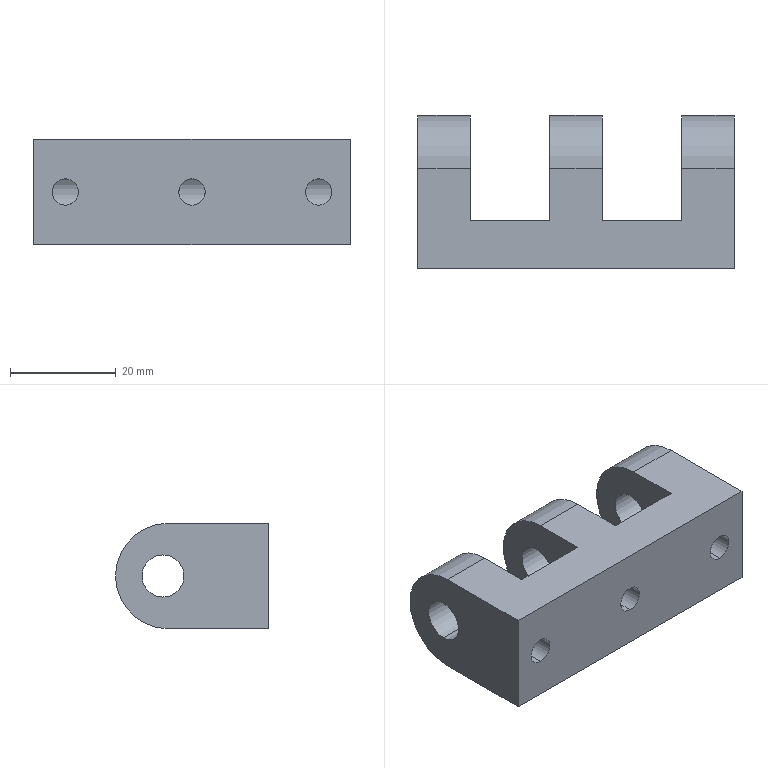Part | SolidWorks | features BaseBody 1 | 1 solid | 26 faces | box 60 x 29 x 20 mm | volume 19050 mm3 | cylinder 15 | plane 11 | commonest cylinder face diameters 5 x6 8 x6 20 x3
STEP:
#1=CARTESIAN_POINT('',(-24.,16.878,-2.5));
#2=VERTEX_POINT('',#1);
#3=CARTESIAN_POINT('',(-24.,16.878,2.5));
#4=VERTEX_POINT('',#3);
#5=CARTESIAN_POINT('',(-24.,16.878,-2.5));
#6=CARTESIAN_POINT('',(-24.17,16.878,-2.5));
#7=CARTESIAN_POINT('',(-24.337,16.864,-2.483));
#8=CARTESIAN_POINT('',(-24.662,16.812,-2.417));
#9=CARTESIAN_POINT('',(-24.822,16.774,-2.367));
#10=CARTESIAN_POINT('',(-25.27,16.641,-2.178));
#11=CARTESIAN_POINT('',(-25.539,16.524,-1.996));
#12=CARTESIAN_POINT('',(-25.876,16.358,-1.66));
#13=CARTESIAN_POINT('',(-25.98,16.304,-1.535));
#14=CARTESIAN_POINT('',(-26.16,16.204,-1.269));
#15=CARTESIAN_POINT('',(-26.237,16.159,-1.128));
#16=CARTESIAN_POINT('',(-26.365,16.083,-0.8272));
#17=CARTESIAN_POINT('',(-26.415,16.052,-0.6657));
#18=CARTESIAN_POINT('',(-26.482,16.011,-0.3399));
#19=CARTESIAN_POINT('',(-26.5,16.,-0.1739));
#20=CARTESIAN_POINT('',(-26.5,16.,0.1647));
#21=CARTESIAN_POINT('',(-26.483,16.011,0.3339));
#22=CARTESIAN_POINT('',(-26.417,16.052,0.6609));
#23=CARTESIAN_POINT('',(-26.367,16.082,0.8221));
#24=CARTESIAN_POINT('',(-26.175,16.196,1.276));
#25=CARTESIAN_POINT('',(-25.989,16.303,1.547));
#26=CARTESIAN_POINT('',(-25.652,16.469,1.883));
#27=CARTESIAN_POINT('',(-25.527,16.526,1.986));
#28=CARTESIAN_POINT('',(-25.262,16.634,2.164));
#29=CARTESIAN_POINT('',(-25.122,16.685,2.24));
#30=CARTESIAN_POINT('',(-24.823,16.774,2.366));
#31=CARTESIAN_POINT('',(-24.663,16.812,2.416));
#32=CARTESIAN_POINT('',(-24.337,16.863,2.483));
#33=CARTESIAN_POINT('',(-24.171,16.878,2.5));
#34=CARTESIAN_POINT('',(-24.,16.878,2.5));
#35=B_SPLINE_CURVE_WITH_KNOTS('',3,(#5,#6,#7,#8,#9,#10,#11,#12,#13,#14,#15,#16,#17,#18,#19,#20,#21,#22,#23,#24,#25,#26,#27,#28,#29,#30,#31,#32,#33,#34),.UNSPECIFIED.,.F.,.F.,(4,2,2,2,2,2,2,2,2,2,2,2,2,2,4),(0.,0.0005024,0.001005,0.00201,0.002512,0.003015,0.003517,0.004019,0.004522,0.005024,0.006029,0.006532,0.007034,0.007536,0.008039),.UNSPECIFIED.);
#36=EDGE_CURVE('',#2,#4,#35,.T.);
#37=ORIENTED_EDGE('',*,*,#36,.F.);
#38=CARTESIAN_POINT('',(-24.,16.878,2.5));
#39=CARTESIAN_POINT('',(-23.83,16.878,2.5));
#40=CARTESIAN_POINT('',(-23.663,16.864,2.483));
#41=CARTESIAN_POINT('',(-23.338,16.812,2.417));
#42=CARTESIAN_POINT('',(-23.178,16.774,2.367));
#43=CARTESIAN_POINT('',(-22.73,16.641,2.178));
#44=CARTESIAN_POINT('',(-22.461,16.524,1.996));
#45=CARTESIAN_POINT('',(-22.124,16.358,1.66));
#46=CARTESIAN_POINT('',(-22.02,16.304,1.535));
#47=CARTESIAN_POINT('',(-21.84,16.204,1.269));
#48=CARTESIAN_POINT('',(-21.763,16.159,1.128));
#49=CARTESIAN_POINT('',(-21.635,16.083,0.8272));
#50=CARTESIAN_POINT('',(-21.585,16.052,0.6657));
#51=CARTESIAN_POINT('',(-21.518,16.011,0.3399));
#52=CARTESIAN_POINT('',(-21.5,16.,0.1739));
#53=CARTESIAN_POINT('',(-21.5,16.,-0.1647));
#54=CARTESIAN_POINT('',(-21.517,16.011,-0.3339));
#55=CARTESIAN_POINT('',(-21.583,16.052,-0.6609));
#56=CARTESIAN_POINT('',(-21.633,16.082,-0.8221));
#57=CARTESIAN_POINT('',(-21.825,16.196,-1.276));
#58=CARTESIAN_POINT('',(-22.011,16.303,-1.547));
#59=CARTESIAN_POINT('',(-22.348,16.469,-1.883));
#60=CARTESIAN_POINT('',(-22.473,16.526,-1.986));
#61=CARTESIAN_POINT('',(-22.738,16.634,-2.164));
#62=CARTESIAN_POINT('',(-22.878,16.685,-2.24));
#63=CARTESIAN_POINT('',(-23.177,16.774,-2.366));
#64=CARTESIAN_POINT('',(-23.337,16.812,-2.416));
#65=CARTESIAN_POINT('',(-23.663,16.863,-2.483));
#66=CARTESIAN_POINT('',(-23.83,16.878,-2.5));
#67=CARTESIAN_POINT('',(-24.,16.878,-2.5));
#68=B_SPLINE_CURVE_WITH_KNOTS('',3,(#38,#39,#40,#41,#42,#43,#44,#45,#46,#47,#48,#49,#50,#51,#52,#53,#54,#55,#56,#57,#58,#59,#60,#61,#62,#63,#64,#65,#66,#67),.UNSPECIFIED.,.F.,.F.,(4,2,2,2,2,2,2,2,2,2,2,2,2,2,4),(0.008039,0.00854,0.009042,0.01004,0.01055,0.01105,0.01155,0.01205,0.01255,0.01305,0.01406,0.01456,0.01506,0.01556,0.01606),.UNSPECIFIED.);
#69=EDGE_CURVE('',#4,#2,#68,.T.);
#70=ORIENTED_EDGE('',*,*,#69,.F.);
#71=EDGE_LOOP('',(#37,#70));
#72=FACE_BOUND('',#71,.T.);
#73=CARTESIAN_POINT('',(-30.,20.,4.));
#74=VERTEX_POINT('',#73);
#75=CARTESIAN_POINT('',(-30.,20.,-4.));
#76=VERTEX_POINT('',#75);
#77=CARTESIAN_POINT('',(-30.,20.,0.));
#78=DIRECTION('',(1.,0.,0.));
#79=DIRECTION('',(0.,0.,-1.));
#80=AXIS2_PLACEMENT_3D('',#77,#78,#79);
#81=CIRCLE('',#80,4.);
#82=EDGE_CURVE('',#74,#76,#81,.T.);
#83=ORIENTED_EDGE('',*,*,#82,.F.);
#84=CARTESIAN_POINT('',(-20.,20.,4.));
#85=VERTEX_POINT('',#84);
#86=CARTESIAN_POINT('',(-30.,20.,4.));
#87=DIRECTION('',(1.,0.,0.));
#88=VECTOR('',#87,1000.);
#89=LINE('',#86,#88);
#90=EDGE_CURVE('',#74,#85,#89,.T.);
#91=ORIENTED_EDGE('',*,*,#90,.T.);
#92=CARTESIAN_POINT('',(-20.,20.,-4.));
#93=VERTEX_POINT('',#92);
#94=CARTESIAN_POINT('',(-20.,20.,0.));
#95=DIRECTION('',(-1.,0.,0.));
#96=DIRECTION('',(0.,0.,1.));
#97=AXIS2_PLACEMENT_3D('',#94,#95,#96);
#98=CIRCLE('',#97,4.);
#99=EDGE_CURVE('',#93,#85,#98,.T.);
#100=ORIENTED_EDGE('',*,*,#99,.F.);
#101=CARTESIAN_POINT('',(-30.,20.,-4.));
#102=DIRECTION('',(1.,0.,0.));
#103=VECTOR('',#102,1000.);
#104=LINE('',#101,#103);
#105=EDGE_CURVE('',#76,#93,#104,.T.);
#106=ORIENTED_EDGE('',*,*,#105,.F.);
#107=EDGE_LOOP('',(#83,#91,#100,#106));
#108=FACE_OUTER_BOUND('',#107,.T.);
#109=CARTESIAN_POINT('',(-30.,20.,0.));
#110=DIRECTION('',(1.,0.,0.));
#111=DIRECTION('',(0.,0.,-1.));
#112=AXIS2_PLACEMENT_3D('',#109,#110,#111);
#113=CYLINDRICAL_SURFACE('',#112,4.);
#114=ADVANCED_FACE('',(#72,#108),#113,.F.);
#115=CARTESIAN_POINT('',(0.,16.878,-2.5));
#116=VERTEX_POINT('',#115);
#117=CARTESIAN_POINT('',(0.,16.878,2.5));
#118=VERTEX_POINT('',#117);
#119=CARTESIAN_POINT('',(0.,16.878,-2.5));
#120=CARTESIAN_POINT('',(-0.1704,16.878,-2.5));
#121=CARTESIAN_POINT('',(-0.3367,16.864,-2.483));
#122=CARTESIAN_POINT('',(-0.6617,16.812,-2.417));
#123=CARTESIAN_POINT('',(-0.8216,16.774,-2.367));
#124=CARTESIAN_POINT('',(-1.27,16.641,-2.178));
#125=CARTESIAN_POINT('',(-1.539,16.524,-1.996));
#126=CARTESIAN_POINT('',(-1.876,16.358,-1.66));
#127=CARTESIAN_POINT('',(-1.98,16.304,-1.535));
#128=CARTESIAN_POINT('',(-2.16,16.204,-1.269));
#129=CARTESIAN_POINT('',(-2.237,16.159,-1.128));
#130=CARTESIAN_POINT('',(-2.365,16.083,-0.8272));
#131=CARTESIAN_POINT('',(-2.415,16.052,-0.6657));
#132=CARTESIAN_POINT('',(-2.482,16.011,-0.3399));
#133=CARTESIAN_POINT('',(-2.5,16.,-0.1739));
#134=CARTESIAN_POINT('',(-2.5,16.,0.1647));
#135=CARTESIAN_POINT('',(-2.483,16.011,0.3339));
#136=CARTESIAN_POINT('',(-2.417,16.052,0.6609));
#137=CARTESIAN_POINT('',(-2.367,16.082,0.8221));
#138=CARTESIAN_POINT('',(-2.175,16.196,1.276));
#139=CARTESIAN_POINT('',(-1.989,16.303,1.547));
#140=CARTESIAN_POINT('',(-1.652,16.469,1.883));
#141=CARTESIAN_POINT('',(-1.527,16.526,1.986));
#142=CARTESIAN_POINT('',(-1.262,16.634,2.164));
#143=CARTESIAN_POINT('',(-1.122,16.685,2.24));
#144=CARTESIAN_POINT('',(-0.8234,16.774,2.366));
#145=CARTESIAN_POINT('',(-0.6631,16.812,2.416));
#146=CARTESIAN_POINT('',(-0.3373,16.863,2.483));
#147=CARTESIAN_POINT('',(-0.1708,16.878,2.5));
#148=CARTESIAN_POINT('',(0.,16.878,2.5));
#149=B_SPLINE_CURVE_WITH_KNOTS('',3,(#119,#120,#121,#122,#123,#124,#125,#126,#127,#128,#129,#130,#131,#132,#133,#134,#135,#136,#137,#138,#139,#140,#141,#142,#143,#144,#145,#146,#147,#148),.UNSPECIFIED.,.F.,.F.,(4,2,2,2,2,2,2,2,2,2,2,2,2,2,4),(0.,0.0005024,0.001005,0.00201,0.002512,0.003015,0.003517,0.004019,0.004522,0.005024,0.006029,0.006532,0.007034,0.007536,0.008039),.UNSPECIFIED.);
#150=EDGE_CURVE('',#116,#118,#149,.T.);
#151=ORIENTED_EDGE('',*,*,#150,.F.);
#152=CARTESIAN_POINT('',(0.,16.878,2.5));
#153=CARTESIAN_POINT('',(0.1704,16.878,2.5));
#154=CARTESIAN_POINT('',(0.3367,16.864,2.483));
#155=CARTESIAN_POINT('',(0.6617,16.812,2.417));
#156=CARTESIAN_POINT('',(0.8216,16.774,2.367));
#157=CARTESIAN_POINT('',(1.27,16.641,2.178));
#158=CARTESIAN_POINT('',(1.539,16.524,1.996));
#159=CARTESIAN_POINT('',(1.876,16.358,1.66));
#160=CARTESIAN_POINT('',(1.98,16.304,1.535));
#161=CARTESIAN_POINT('',(2.16,16.204,1.269));
#162=CARTESIAN_POINT('',(2.237,16.159,1.128));
#163=CARTESIAN_POINT('',(2.365,16.083,0.8272));
#164=CARTESIAN_POINT('',(2.415,16.052,0.6657));
#165=CARTESIAN_POINT('',(2.482,16.011,0.3399));
#166=CARTESIAN_POINT('',(2.5,16.,0.1739));
#167=CARTESIAN_POINT('',(2.5,16.,-0.1647));
#168=CARTESIAN_POINT('',(2.483,16.011,-0.3339));
#169=CARTESIAN_POINT('',(2.417,16.052,-0.6609));
#170=CARTESIAN_POINT('',(2.367,16.082,-0.8221));
#171=CARTESIAN_POINT('',(2.175,16.196,-1.276));
#172=CARTESIAN_POINT('',(1.989,16.303,-1.547));
#173=CARTESIAN_POINT('',(1.652,16.469,-1.883));
#174=CARTESIAN_POINT('',(1.527,16.526,-1.986));
#175=CARTESIAN_POINT('',(1.262,16.634,-2.164));
#176=CARTESIAN_POINT('',(1.122,16.685,-2.24));
#177=CARTESIAN_POINT('',(0.8234,16.774,-2.366));
#178=CARTESIAN_POINT('',(0.6631,16.812,-2.416));
#179=CARTESIAN_POINT('',(0.3373,16.863,-2.483));
#180=CARTESIAN_POINT('',(0.1701,16.878,-2.5));
#181=CARTESIAN_POINT('',(0.,16.878,-2.5));
#182=B_SPLINE_CURVE_WITH_KNOTS('',3,(#152,#153,#154,#155,#156,#157,#158,#159,#160,#161,#162,#163,#164,#165,#166,#167,#168,#169,#170,#171,#172,#173,#174,#175,#176,#177,#178,#179,#180,#181),.UNSPECIFIED.,.F.,.F.,(4,2,2,2,2,2,2,2,2,2,2,2,2,2,4),(0.008039,0.00854,0.009042,0.01004,0.01055,0.01105,0.01155,0.01205,0.01255,0.01305,0.01406,0.01456,0.01506,0.01556,0.01606),.UNSPECIFIED.);
#183=EDGE_CURVE('',#118,#116,#182,.T.);
#184=ORIENTED_EDGE('',*,*,#183,.F.);
#185=EDGE_LOOP('',(#151,#184));
#186=FACE_BOUND('',#185,.T.);
#187=CARTESIAN_POINT('',(-5.,20.,4.));
#188=VERTEX_POINT('',#187);
#189=CARTESIAN_POINT('',(-5.,20.,-4.));
#190=VERTEX_POINT('',#189);
#191=CARTESIAN_POINT('',(-5.,20.,0.));
#192=DIRECTION('',(1.,0.,0.));
#193=DIRECTION('',(0.,1.,0.));
#194=AXIS2_PLACEMENT_3D('',#191,#192,#193);
#195=CIRCLE('',#194,4.);
#196=EDGE_CURVE('',#188,#190,#195,.T.);
#197=ORIENTED_EDGE('',*,*,#196,.F.);
#198=CARTESIAN_POINT('',(5.,20.,4.));
#199=VERTEX_POINT('',#198);
#200=CARTESIAN_POINT('',(-30.,20.,4.));
#201=DIRECTION('',(1.,0.,0.));
#202=VECTOR('',#201,1000.);
#203=LINE('',#200,#202);
#204=EDGE_CURVE('',#188,#199,#203,.T.);
#205=ORIENTED_EDGE('',*,*,#204,.T.);
#206=CARTESIAN_POINT('',(5.,20.,-4.));
#207=VERTEX_POINT('',#206);
#208=CARTESIAN_POINT('',(5.,20.,0.));
#209=DIRECTION('',(-1.,0.,0.));
#210=DIRECTION('',(0.,0.,1.));
#211=AXIS2_PLACEMENT_3D('',#208,#209,#210);
#212=CIRCLE('',#211,4.);
#213=EDGE_CURVE('',#207,#199,#212,.T.);
#214=ORIENTED_EDGE('',*,*,#213,.F.);
#215=CARTESIAN_POINT('',(-30.,20.,-4.));
#216=DIRECTION('',(1.,0.,0.));
#217=VECTOR('',#216,1000.);
#218=LINE('',#215,#217);
#219=EDGE_CURVE('',#190,#207,#218,.T.);
#220=ORIENTED_EDGE('',*,*,#219,.F.);
#221=EDGE_LOOP('',(#197,#205,#214,#220));
#222=FACE_OUTER_BOUND('',#221,.T.);
#223=CARTESIAN_POINT('',(-30.,20.,0.));
#224=DIRECTION('',(1.,0.,0.));
#225=DIRECTION('',(0.,0.,-1.));
#226=AXIS2_PLACEMENT_3D('',#223,#224,#225);
#227=CYLINDRICAL_SURFACE('',#226,4.);
#228=ADVANCED_FACE('',(#186,#222),#227,.F.);
#229=CARTESIAN_POINT('',(24.,16.878,-2.5));
#230=VERTEX_POINT('',#229);
#231=CARTESIAN_POINT('',(24.,16.878,2.5));
#232=VERTEX_POINT('',#231);
#233=CARTESIAN_POINT('',(24.,16.878,-2.5));
#234=CARTESIAN_POINT('',(23.83,16.878,-2.5));
#235=CARTESIAN_POINT('',(23.663,16.864,-2.483));
#236=CARTESIAN_POINT('',(23.338,16.812,-2.417));
#237=CARTESIAN_POINT('',(23.178,16.774,-2.367));
#238=CARTESIAN_POINT('',(22.73,16.641,-2.178));
#239=CARTESIAN_POINT('',(22.461,16.524,-1.996));
#240=CARTESIAN_POINT('',(22.124,16.358,-1.66));
#241=CARTESIAN_POINT('',(22.02,16.304,-1.535));
#242=CARTESIAN_POINT('',(21.84,16.204,-1.269));
#243=CARTESIAN_POINT('',(21.763,16.159,-1.128));
#244=CARTESIAN_POINT('',(21.635,16.083,-0.8272));
#245=CARTESIAN_POINT('',(21.585,16.052,-0.6657));
#246=CARTESIAN_POINT('',(21.518,16.011,-0.3399));
#247=CARTESIAN_POINT('',(21.5,16.,-0.1739));
#248=CARTESIAN_POINT('',(21.5,16.,0.1647));
#249=CARTESIAN_POINT('',(21.517,16.011,0.3339));
#250=CARTESIAN_POINT('',(21.583,16.052,0.6609));
#251=CARTESIAN_POINT('',(21.633,16.082,0.8221));
#252=CARTESIAN_POINT('',(21.825,16.196,1.276));
#253=CARTESIAN_POINT('',(22.011,16.303,1.547));
#254=CARTESIAN_POINT('',(22.348,16.469,1.883));
#255=CARTESIAN_POINT('',(22.473,16.526,1.986));
#256=CARTESIAN_POINT('',(22.738,16.634,2.164));
#257=CARTESIAN_POINT('',(22.878,16.685,2.24));
#258=CARTESIAN_POINT('',(23.177,16.774,2.366));
#259=CARTESIAN_POINT('',(23.337,16.812,2.416));
#260=CARTESIAN_POINT('',(23.663,16.863,2.483));
#261=CARTESIAN_POINT('',(23.829,16.878,2.5));
#262=CARTESIAN_POINT('',(24.,16.878,2.5));
#263=B_SPLINE_CURVE_WITH_KNOTS('',3,(#233,#234,#235,#236,#237,#238,#239,#240,#241,#242,#243,#244,#245,#246,#247,#248,#249,#250,#251,#252,#253,#254,#255,#256,#257,#258,#259,#260,#261,#262),.UNSPECIFIED.,.F.,.F.,(4,2,2,2,2,2,2,2,2,2,2,2,2,2,4),(0.,0.0005024,0.001005,0.00201,0.002512,0.003015,0.003517,0.004019,0.004522,0.005024,0.006029,0.006532,0.007034,0.007536,0.008039),.UNSPECIFIED.);
#264=EDGE_CURVE('',#230,#232,#263,.T.);
#265=ORIENTED_EDGE('',*,*,#264,.F.);
#266=CARTESIAN_POINT('',(24.,16.878,2.5));
#267=CARTESIAN_POINT('',(24.17,16.878,2.5));
#268=CARTESIAN_POINT('',(24.337,16.864,2.483));
#269=CARTESIAN_POINT('',(24.662,16.812,2.417));
#270=CARTESIAN_POINT('',(24.822,16.774,2.367));
#271=CARTESIAN_POINT('',(25.27,16.641,2.178));
#272=CARTESIAN_POINT('',(25.539,16.524,1.996));
#273=CARTESIAN_POINT('',(25.876,16.358,1.66));
#274=CARTESIAN_POINT('',(25.98,16.304,1.535));
#275=CARTESIAN_POINT('',(26.16,16.204,1.269));
#276=CARTESIAN_POINT('',(26.237,16.159,1.128));
#277=CARTESIAN_POINT('',(26.365,16.083,0.8272));
#278=CARTESIAN_POINT('',(26.415,16.052,0.6657));
#279=CARTESIAN_POINT('',(26.482,16.011,0.3399));
#280=CARTESIAN_POINT('',(26.5,16.,0.1739));
#281=CARTESIAN_POINT('',(26.5,16.,-0.1647));
#282=CARTESIAN_POINT('',(26.483,16.011,-0.3339));
#283=CARTESIAN_POINT('',(26.417,16.052,-0.6609));
#284=CARTESIAN_POINT('',(26.367,16.082,-0.8221));
#285=CARTESIAN_POINT('',(26.175,16.196,-1.276));
#286=CARTESIAN_POINT('',(25.989,16.303,-1.547));
#287=CARTESIAN_POINT('',(25.652,16.469,-1.883));
#288=CARTESIAN_POINT('',(25.527,16.526,-1.986));
#289=CARTESIAN_POINT('',(25.262,16.634,-2.164));
#290=CARTESIAN_POINT('',(25.122,16.685,-2.24));
#291=CARTESIAN_POINT('',(24.823,16.774,-2.366));
#292=CARTESIAN_POINT('',(24.663,16.812,-2.416));
#293=CARTESIAN_POINT('',(24.337,16.863,-2.483));
#294=CARTESIAN_POINT('',(24.17,16.878,-2.5));
#295=CARTESIAN_POINT('',(24.,16.878,-2.5));
#296=B_SPLINE_CURVE_WITH_KNOTS('',3,(#266,#267,#268,#269,#270,#271,#272,#273,#274,#275,#276,#277,#278,#279,#280,#281,#282,#283,#284,#285,#286,#287,#288,#289,#290,#291,#292,#293,#294,#295),.UNSPECIFIED.,.F.,.F.,(4,2,2,2,2,2,2,2,2,2,2,2,2,2,4),(0.008039,0.00854,0.009042,0.01004,0.01055,0.01105,0.01155,0.01205,0.01255,0.01305,0.01406,0.01456,0.01506,0.01556,0.01606),.UNSPECIFIED.);
#297=EDGE_CURVE('',#232,#230,#296,.T.);
#298=ORIENTED_EDGE('',*,*,#297,.F.);
#299=EDGE_LOOP('',(#265,#298));
#300=FACE_BOUND('',#299,.T.);
#301=CARTESIAN_POINT('',(20.,20.,4.));
#302=VERTEX_POINT('',#301);
#303=CARTESIAN_POINT('',(20.,20.,-4.));
#304=VERTEX_POINT('',#303);
#305=CARTESIAN_POINT('',(20.,20.,0.));
#306=DIRECTION('',(1.,0.,0.));
#307=DIRECTION('',(0.,1.,0.));
#308=AXIS2_PLACEMENT_3D('',#305,#306,#307);
#309=CIRCLE('',#308,4.);
#310=EDGE_CURVE('',#302,#304,#309,.T.);
#311=ORIENTED_EDGE('',*,*,#310,.F.);
#312=CARTESIAN_POINT('',(30.,20.,4.));
#313=VERTEX_POINT('',#312);
#314=CARTESIAN_POINT('',(-30.,20.,4.));
#315=DIRECTION('',(1.,0.,0.));
#316=VECTOR('',#315,1000.);
#317=LINE('',#314,#316);
#318=EDGE_CURVE('',#302,#313,#317,.T.);
#319=ORIENTED_EDGE('',*,*,#318,.T.);
#320=CARTESIAN_POINT('',(30.,20.,-4.));
#321=VERTEX_POINT('',#320);
#322=CARTESIAN_POINT('',(30.,20.,0.));
#323=DIRECTION('',(1.,0.,0.));
#324=DIRECTION('',(0.,0.,-1.));
#325=AXIS2_PLACEMENT_3D('',#322,#323,#324);
#326=CIRCLE('',#325,4.);
#327=EDGE_CURVE('',#313,#321,#326,.T.);
#328=ORIENTED_EDGE('',*,*,#327,.T.);
#329=CARTESIAN_POINT('',(-30.,20.,-4.));
#330=DIRECTION('',(1.,0.,0.));
#331=VECTOR('',#330,1000.);
#332=LINE('',#329,#331);
#333=EDGE_CURVE('',#304,#321,#332,.T.);
#334=ORIENTED_EDGE('',*,*,#333,.F.);
#335=EDGE_LOOP('',(#311,#319,#328,#334));
#336=FACE_OUTER_BOUND('',#335,.T.);
#337=CARTESIAN_POINT('',(-30.,20.,0.));
#338=DIRECTION('',(1.,0.,0.));
#339=DIRECTION('',(0.,0.,-1.));
#340=AXIS2_PLACEMENT_3D('',#337,#338,#339);
#341=CYLINDRICAL_SURFACE('',#340,4.);
#342=ADVANCED_FACE('',(#300,#336),#341,.F.);
#343=ORIENTED_EDGE('',*,*,#36,.T.);
#344=CARTESIAN_POINT('',(-24.,0.,2.5));
#345=VERTEX_POINT('',#344);
#346=CARTESIAN_POINT('',(-24.,0.,2.5));
#347=DIRECTION('',(0.,-1.,0.));
#348=VECTOR('',#347,1000.);
#349=LINE('',#346,#348);
#350=EDGE_CURVE('',#4,#345,#349,.T.);
#351=ORIENTED_EDGE('',*,*,#350,.T.);
#352=CARTESIAN_POINT('',(-24.,0.,-2.5));
#353=VERTEX_POINT('',#352);
#354=CARTESIAN_POINT('',(-24.,0.,0.));
#355=DIRECTION('',(0.,-1.,0.));
#356=DIRECTION('',(0.,0.,-1.));
#357=AXIS2_PLACEMENT_3D('',#354,#355,#356);
#358=CIRCLE('',#357,2.5);
#359=EDGE_CURVE('',#345,#353,#358,.T.);
#360=ORIENTED_EDGE('',*,*,#359,.T.);
#361=CARTESIAN_POINT('',(-24.,0.,-2.5));
#362=DIRECTION('',(0.,-1.,0.));
#363=VECTOR('',#362,1000.);
#364=LINE('',#361,#363);
#365=EDGE_CURVE('',#2,#353,#364,.T.);
#366=ORIENTED_EDGE('',*,*,#365,.F.);
#367=EDGE_LOOP('',(#343,#351,#360,#366));
#368=FACE_OUTER_BOUND('',#367,.T.);
#369=CARTESIAN_POINT('',(-24.,0.,0.));
#370=DIRECTION('',(0.,-1.,0.));
#371=DIRECTION('',(0.,0.,-1.));
#372=AXIS2_PLACEMENT_3D('',#369,#370,#371);
#373=CYLINDRICAL_SURFACE('',#372,2.5);
#374=ADVANCED_FACE('',(#368),#373,.F.);
#375=ORIENTED_EDGE('',*,*,#150,.T.);
#376=CARTESIAN_POINT('',(0.,0.,2.5));
#377=VERTEX_POINT('',#376);
#378=CARTESIAN_POINT('',(0.,0.,2.5));
#379=DIRECTION('',(0.,-1.,0.));
#380=VECTOR('',#379,1000.);
#381=LINE('',#378,#380);
#382=EDGE_CURVE('',#118,#377,#381,.T.);
#383=ORIENTED_EDGE('',*,*,#382,.T.);
#384=CARTESIAN_POINT('',(0.,0.,-2.5));
#385=VERTEX_POINT('',#384);
#386=CARTESIAN_POINT('',(0.,0.,0.));
#387=DIRECTION('',(0.,-1.,0.));
#388=DIRECTION('',(0.,0.,-1.));
#389=AXIS2_PLACEMENT_3D('',#386,#387,#388);
#390=CIRCLE('',#389,2.5);
#391=EDGE_CURVE('',#377,#385,#390,.T.);
#392=ORIENTED_EDGE('',*,*,#391,.T.);
#393=CARTESIAN_POINT('',(0.,0.,-2.5));
#394=DIRECTION('',(0.,-1.,0.));
#395=VECTOR('',#394,1000.);
#396=LINE('',#393,#395);
#397=EDGE_CURVE('',#116,#385,#396,.T.);
#398=ORIENTED_EDGE('',*,*,#397,.F.);
#399=EDGE_LOOP('',(#375,#383,#392,#398));
#400=FACE_OUTER_BOUND('',#399,.T.);
#401=CARTESIAN_POINT('',(0.,0.,0.));
#402=DIRECTION('',(0.,-1.,0.));
#403=DIRECTION('',(0.,0.,-1.));
#404=AXIS2_PLACEMENT_3D('',#401,#402,#403);
#405=CYLINDRICAL_SURFACE('',#404,2.5);
#406=ADVANCED_FACE('',(#400),#405,.F.);
#407=ORIENTED_EDGE('',*,*,#264,.T.);
#408=CARTESIAN_POINT('',(24.,0.,2.5));
#409=VERTEX_POINT('',#408);
#410=CARTESIAN_POINT('',(24.,0.,2.5));
#411=DIRECTION('',(0.,-1.,0.));
#412=VECTOR('',#411,1000.);
#413=LINE('',#410,#412);
#414=EDGE_CURVE('',#232,#409,#413,.T.);
#415=ORIENTED_EDGE('',*,*,#414,.T.);
#416=CARTESIAN_POINT('',(24.,0.,-2.5));
#417=VERTEX_POINT('',#416);
#418=CARTESIAN_POINT('',(24.,0.,0.));
#419=DIRECTION('',(0.,-1.,0.));
#420=DIRECTION('',(0.,0.,-1.));
#421=AXIS2_PLACEMENT_3D('',#418,#419,#420);
#422=CIRCLE('',#421,2.5);
#423=EDGE_CURVE('',#409,#417,#422,.T.);
#424=ORIENTED_EDGE('',*,*,#423,.T.);
#425=CARTESIAN_POINT('',(24.,0.,-2.5));
#426=DIRECTION('',(0.,-1.,0.));
#427=VECTOR('',#426,1000.);
#428=LINE('',#425,#427);
#429=EDGE_CURVE('',#230,#417,#428,.T.);
#430=ORIENTED_EDGE('',*,*,#429,.F.);
#431=EDGE_LOOP('',(#407,#415,#424,#430));
#432=FACE_OUTER_BOUND('',#431,.T.);
#433=CARTESIAN_POINT('',(24.,0.,0.));
#434=DIRECTION('',(0.,-1.,0.));
#435=DIRECTION('',(0.,0.,-1.));
#436=AXIS2_PLACEMENT_3D('',#433,#434,#435);
#437=CYLINDRICAL_SURFACE('',#436,2.5);
#438=ADVANCED_FACE('',(#432),#437,.F.);
#439=CARTESIAN_POINT('',(20.,19.,-10.));
#440=VERTEX_POINT('',#439);
#441=CARTESIAN_POINT('',(30.,19.,-10.));
#442=VERTEX_POINT('',#441);
#443=CARTESIAN_POINT('',(30.,19.,-10.));
#444=DIRECTION('',(1.,0.,0.));
#445=VECTOR('',#444,1000.);
#446=LINE('',#443,#445);
#447=EDGE_CURVE('',#440,#442,#446,.T.);
#448=ORIENTED_EDGE('',*,*,#447,.F.);
#449=CARTESIAN_POINT('',(20.,19.,10.));
#450=VERTEX_POINT('',#449);
#451=CARTESIAN_POINT('',(20.,19.,0.));
#452=DIRECTION('',(-1.,0.,0.));
#453=DIRECTION('',(0.,1.,0.));
#454=AXIS2_PLACEMENT_3D('',#451,#452,#453);
#455=CIRCLE('',#454,10.);
#456=EDGE_CURVE('',#450,#440,#455,.T.);
#457=ORIENTED_EDGE('',*,*,#456,.F.);
#458=CARTESIAN_POINT('',(30.,19.,10.));
#459=VERTEX_POINT('',#458);
#460=CARTESIAN_POINT('',(20.,19.,10.));
#461=DIRECTION('',(-1.,0.,0.));
#462=VECTOR('',#461,1000.);
#463=LINE('',#460,#462);
#464=EDGE_CURVE('',#459,#450,#463,.T.);
#465=ORIENTED_EDGE('',*,*,#464,.F.);
#466=CARTESIAN_POINT('',(30.,19.,0.));
#467=DIRECTION('',(1.,0.,0.));
#468=DIRECTION('',(0.,0.,1.));
#469=AXIS2_PLACEMENT_3D('',#466,#467,#468);
#470=CIRCLE('',#469,10.);
#471=EDGE_CURVE('',#442,#459,#470,.T.);
#472=ORIENTED_EDGE('',*,*,#471,.F.);
#473=EDGE_LOOP('',(#448,#457,#465,#472));
#474=FACE_OUTER_BOUND('',#473,.T.);
#475=CARTESIAN_POINT('',(0.,19.,0.));
#476=DIRECTION('',(1.,0.,0.));
#477=DIRECTION('',(0.,0.,-1.));
#478=AXIS2_PLACEMENT_3D('',#475,#476,#477);
#479=CYLINDRICAL_SURFACE('',#478,10.);
#480=ADVANCED_FACE('',(#474),#479,.T.);
#481=CARTESIAN_POINT('',(5.,19.,10.));
#482=VERTEX_POINT('',#481);
#483=CARTESIAN_POINT('',(-5.,19.,10.));
#484=VERTEX_POINT('',#483);
#485=CARTESIAN_POINT('',(-5.,19.,10.));
#486=DIRECTION('',(-1.,0.,0.));
#487=VECTOR('',#486,1000.);
#488=LINE('',#485,#487);
#489=EDGE_CURVE('',#482,#484,#488,.T.);
#490=ORIENTED_EDGE('',*,*,#489,.F.);
#491=CARTESIAN_POINT('',(5.,19.,-10.));
#492=VERTEX_POINT('',#491);
#493=CARTESIAN_POINT('',(5.,19.,0.));
#494=DIRECTION('',(1.,0.,0.));
#495=DIRECTION('',(0.,0.,1.));
#496=AXIS2_PLACEMENT_3D('',#493,#494,#495);
#497=CIRCLE('',#496,10.);
#498=EDGE_CURVE('',#492,#482,#497,.T.);
#499=ORIENTED_EDGE('',*,*,#498,.F.);
#500=CARTESIAN_POINT('',(-5.,19.,-10.));
#501=VERTEX_POINT('',#500);
#502=CARTESIAN_POINT('',(5.,19.,-10.));
#503=DIRECTION('',(1.,0.,0.));
#504=VECTOR('',#503,1000.);
#505=LINE('',#502,#504);
#506=EDGE_CURVE('',#501,#492,#505,.T.);
#507=ORIENTED_EDGE('',*,*,#506,.F.);
#508=CARTESIAN_POINT('',(-5.,19.,0.));
#509=DIRECTION('',(-1.,0.,0.));
#510=DIRECTION('',(0.,1.,0.));
#511=AXIS2_PLACEMENT_3D('',#508,#509,#510);
#512=CIRCLE('',#511,10.);
#513=EDGE_CURVE('',#484,#501,#512,.T.);
#514=ORIENTED_EDGE('',*,*,#513,.F.);
#515=EDGE_LOOP('',(#490,#499,#507,#514));
#516=FACE_OUTER_BOUND('',#515,.T.);
#517=CARTESIAN_POINT('',(0.,19.,0.));
#518=DIRECTION('',(-1.,0.,0.));
#519=DIRECTION('',(0.,0.,1.));
#520=AXIS2_PLACEMENT_3D('',#517,#518,#519);
#521=CYLINDRICAL_SURFACE('',#520,10.);
#522=ADVANCED_FACE('',(#516),#521,.T.);
#523=CARTESIAN_POINT('',(-30.,19.,-10.));
#524=VERTEX_POINT('',#523);
#525=CARTESIAN_POINT('',(-20.,19.,-10.));
#526=VERTEX_POINT('',#525);
#527=CARTESIAN_POINT('',(-20.,19.,-10.));
#528=DIRECTION('',(1.,0.,0.));
#529=VECTOR('',#528,1000.);
#530=LINE('',#527,#529);
#531=EDGE_CURVE('',#524,#526,#530,.T.);
#532=ORIENTED_EDGE('',*,*,#531,.F.);
#533=CARTESIAN_POINT('',(-30.,19.,10.));
#534=VERTEX_POINT('',#533);
#535=CARTESIAN_POINT('',(-30.,19.,0.));
#536=DIRECTION('',(-1.,0.,0.));
#537=DIRECTION('',(0.,0.,-1.));
#538=AXIS2_PLACEMENT_3D('',#535,#536,#537);
#539=CIRCLE('',#538,10.);
#540=EDGE_CURVE('',#534,#524,#539,.T.);
#541=ORIENTED_EDGE('',*,*,#540,.F.);
#542=CARTESIAN_POINT('',(-20.,19.,10.));
#543=VERTEX_POINT('',#542);
#544=CARTESIAN_POINT('',(-30.,19.,10.));
#545=DIRECTION('',(-1.,0.,0.));
#546=VECTOR('',#545,1000.);
#547=LINE('',#544,#546);
#548=EDGE_CURVE('',#543,#534,#547,.T.);
#549=ORIENTED_EDGE('',*,*,#548,.F.);
#550=CARTESIAN_POINT('',(-20.,19.,0.));
#551=DIRECTION('',(1.,0.,0.));
#552=DIRECTION('',(0.,0.,1.));
#553=AXIS2_PLACEMENT_3D('',#550,#551,#552);
#554=CIRCLE('',#553,10.);
#555=EDGE_CURVE('',#526,#543,#554,.T.);
#556=ORIENTED_EDGE('',*,*,#555,.F.);
#557=EDGE_LOOP('',(#532,#541,#549,#556));
#558=FACE_OUTER_BOUND('',#557,.T.);
#559=CARTESIAN_POINT('',(0.,19.,0.));
#560=DIRECTION('',(1.,0.,0.));
#561=DIRECTION('',(0.,0.,-1.));
#562=AXIS2_PLACEMENT_3D('',#559,#560,#561);
#563=CYLINDRICAL_SURFACE('',#562,10.);
#564=ADVANCED_FACE('',(#558),#563,.T.);
#565=CARTESIAN_POINT('',(5.,9.,10.));
#566=VERTEX_POINT('',#565);
#567=CARTESIAN_POINT('',(20.,9.,10.));
#568=VERTEX_POINT('',#567);
#569=CARTESIAN_POINT('',(5.,9.,10.));
#570=DIRECTION('',(1.,0.,0.));
#571=VECTOR('',#570,1000.);
#572=LINE('',#569,#571);
#573=EDGE_CURVE('',#566,#568,#572,.T.);
#574=ORIENTED_EDGE('',*,*,#573,.T.);
#575=CARTESIAN_POINT('',(20.,9.,-10.));
#576=VERTEX_POINT('',#575);
#577=CARTESIAN_POINT('',(20.,9.,-10.));
#578=DIRECTION('',(0.,0.,1.));
#579=VECTOR('',#578,1000.);
#580=LINE('',#577,#579);
#581=EDGE_CURVE('',#576,#568,#580,.T.);
#582=ORIENTED_EDGE('',*,*,#581,.F.);
#583=CARTESIAN_POINT('',(5.,9.,-10.));
#584=VERTEX_POINT('',#583);
#585=CARTESIAN_POINT('',(5.,9.,-10.));
#586=DIRECTION('',(1.,0.,0.));
#587=VECTOR('',#586,1000.);
#588=LINE('',#585,#587);
#589=EDGE_CURVE('',#584,#576,#588,.T.);
#590=ORIENTED_EDGE('',*,*,#589,.F.);
#591=CARTESIAN_POINT('',(5.,9.,-10.));
#592=DIRECTION('',(0.,0.,1.));
#593=VECTOR('',#592,1000.);
#594=LINE('',#591,#593);
#595=EDGE_CURVE('',#584,#566,#594,.T.);
#596=ORIENTED_EDGE('',*,*,#595,.T.);
#597=EDGE_LOOP('',(#574,#582,#590,#596));
#598=FACE_OUTER_BOUND('',#597,.T.);
#599=CARTESIAN_POINT('',(5.,9.,-10.));
#600=DIRECTION('',(0.,-1.,0.));
#601=DIRECTION('',(0.,0.,-1.));
#602=AXIS2_PLACEMENT_3D('',#599,#600,#601);
#603=PLANE('',#602);
#604=ADVANCED_FACE('',(#598),#603,.F.);
#605=CARTESIAN_POINT('',(20.,20.,0.));
#606=DIRECTION('',(1.,0.,0.));
#607=DIRECTION('',(0.,1.,0.));
#608=AXIS2_PLACEMENT_3D('',#605,#606,#607);
#609=CIRCLE('',#608,4.);
#610=EDGE_CURVE('',#304,#302,#609,.T.);
#611=ORIENTED_EDGE('',*,*,#610,.T.);
#612=ORIENTED_EDGE('',*,*,#310,.T.);
#613=EDGE_LOOP('',(#611,#612));
#614=FACE_BOUND('',#613,.T.);
#615=CARTESIAN_POINT('',(20.,29.,10.));
#616=DIRECTION('',(0.,1.,0.));
#617=VECTOR('',#616,1000.);
#618=LINE('',#615,#617);
#619=EDGE_CURVE('',#568,#450,#618,.T.);
#620=ORIENTED_EDGE('',*,*,#619,.T.);
#621=ORIENTED_EDGE('',*,*,#456,.T.);
#622=CARTESIAN_POINT('',(20.,29.,-10.));
#623=DIRECTION('',(0.,1.,0.));
#624=VECTOR('',#623,1000.);
#625=LINE('',#622,#624);
#626=EDGE_CURVE('',#576,#440,#625,.T.);
#627=ORIENTED_EDGE('',*,*,#626,.F.);
#628=ORIENTED_EDGE('',*,*,#581,.T.);
#629=EDGE_LOOP('',(#620,#621,#627,#628));
#630=FACE_OUTER_BOUND('',#629,.T.);
#631=CARTESIAN_POINT('',(20.,29.,-10.));
#632=DIRECTION('',(1.,0.,0.));
#633=DIRECTION('',(0.,1.,0.));
#634=AXIS2_PLACEMENT_3D('',#631,#632,#633);
#635=PLANE('',#634);
#636=ADVANCED_FACE('',(#614,#630),#635,.F.);
#637=ORIENTED_EDGE('',*,*,#213,.T.);
#638=CARTESIAN_POINT('',(5.,20.,0.));
#639=DIRECTION('',(-1.,0.,0.));
#640=DIRECTION('',(0.,0.,1.));
#641=AXIS2_PLACEMENT_3D('',#638,#639,#640);
#642=CIRCLE('',#641,4.);
#643=EDGE_CURVE('',#199,#207,#642,.T.);
#644=ORIENTED_EDGE('',*,*,#643,.T.);
#645=EDGE_LOOP('',(#637,#644));
#646=FACE_BOUND('',#645,.T.);
#647=CARTESIAN_POINT('',(5.,29.,-10.));
#648=DIRECTION('',(0.,-1.,0.));
#649=VECTOR('',#648,1000.);
#650=LINE('',#647,#649);
#651=EDGE_CURVE('',#492,#584,#650,.T.);
#652=ORIENTED_EDGE('',*,*,#651,.F.);
#653=ORIENTED_EDGE('',*,*,#498,.T.);
#654=CARTESIAN_POINT('',(5.,29.,10.));
#655=DIRECTION('',(0.,-1.,0.));
#656=VECTOR('',#655,1000.);
#657=LINE('',#654,#656);
#658=EDGE_CURVE('',#482,#566,#657,.T.);
#659=ORIENTED_EDGE('',*,*,#658,.T.);
#660=ORIENTED_EDGE('',*,*,#595,.F.);
#661=EDGE_LOOP('',(#652,#653,#659,#660));
#662=FACE_OUTER_BOUND('',#661,.T.);
#663=CARTESIAN_POINT('',(5.,29.,-10.));
#664=DIRECTION('',(-1.,0.,0.));
#665=DIRECTION('',(0.,0.,1.));
#666=AXIS2_PLACEMENT_3D('',#663,#664,#665);
#667=PLANE('',#666);
#668=ADVANCED_FACE('',(#646,#662),#667,.F.);
#669=CARTESIAN_POINT('',(-20.,9.,10.));
#670=VERTEX_POINT('',#669);
#671=CARTESIAN_POINT('',(-5.,9.,10.));
#672=VERTEX_POINT('',#671);
#673=CARTESIAN_POINT('',(-20.,9.,10.));
#674=DIRECTION('',(1.,0.,0.));
#675=VECTOR('',#674,1000.);
#676=LINE('',#673,#675);
#677=EDGE_CURVE('',#670,#672,#676,.T.);
#678=ORIENTED_EDGE('',*,*,#677,.T.);
#679=CARTESIAN_POINT('',(-5.,9.,-10.));
#680=VERTEX_POINT('',#679);
#681=CARTESIAN_POINT('',(-5.,9.,-10.));
#682=DIRECTION('',(0.,0.,1.));
#683=VECTOR('',#682,1000.);
#684=LINE('',#681,#683);
#685=EDGE_CURVE('',#680,#672,#684,.T.);
#686=ORIENTED_EDGE('',*,*,#685,.F.);
#687=CARTESIAN_POINT('',(-20.,9.,-10.));
#688=VERTEX_POINT('',#687);
#689=CARTESIAN_POINT('',(-20.,9.,-10.));
#690=DIRECTION('',(1.,0.,0.));
#691=VECTOR('',#690,1000.);
#692=LINE('',#689,#691);
#693=EDGE_CURVE('',#688,#680,#692,.T.);
#694=ORIENTED_EDGE('',*,*,#693,.F.);
#695=CARTESIAN_POINT('',(-20.,9.,-10.));
#696=DIRECTION('',(0.,0.,1.));
#697=VECTOR('',#696,1000.);
#698=LINE('',#695,#697);
#699=EDGE_CURVE('',#688,#670,#698,.T.);
#700=ORIENTED_EDGE('',*,*,#699,.T.);
#701=EDGE_LOOP('',(#678,#686,#694,#700));
#702=FACE_OUTER_BOUND('',#701,.T.);
#703=CARTESIAN_POINT('',(-20.,9.,-10.));
#704=DIRECTION('',(0.,-1.,0.));
#705=DIRECTION('',(0.,0.,-1.));
#706=AXIS2_PLACEMENT_3D('',#703,#704,#705);
#707=PLANE('',#706);
#708=ADVANCED_FACE('',(#702),#707,.F.);
#709=CARTESIAN_POINT('',(-5.,20.,0.));
#710=DIRECTION('',(1.,0.,0.));
#711=DIRECTION('',(0.,1.,0.));
#712=AXIS2_PLACEMENT_3D('',#709,#710,#711);
#713=CIRCLE('',#712,4.);
#714=EDGE_CURVE('',#190,#188,#713,.T.);
#715=ORIENTED_EDGE('',*,*,#714,.T.);
#716=ORIENTED_EDGE('',*,*,#196,.T.);
#717=EDGE_LOOP('',(#715,#716));
#718=FACE_BOUND('',#717,.T.);
#719=ORIENTED_EDGE('',*,*,#513,.T.);
#720=CARTESIAN_POINT('',(-5.,29.,-10.));
#721=DIRECTION('',(0.,1.,0.));
#722=VECTOR('',#721,1000.);
#723=LINE('',#720,#722);
#724=EDGE_CURVE('',#680,#501,#723,.T.);
#725=ORIENTED_EDGE('',*,*,#724,.F.);
#726=ORIENTED_EDGE('',*,*,#685,.T.);
#727=CARTESIAN_POINT('',(-5.,29.,10.));
#728=DIRECTION('',(0.,1.,0.));
#729=VECTOR('',#728,1000.);
#730=LINE('',#727,#729);
#731=EDGE_CURVE('',#672,#484,#730,.T.);
#732=ORIENTED_EDGE('',*,*,#731,.T.);
#733=EDGE_LOOP('',(#719,#725,#726,#732));
#734=FACE_OUTER_BOUND('',#733,.T.);
#735=CARTESIAN_POINT('',(-5.,29.,-10.));
#736=DIRECTION('',(1.,0.,0.));
#737=DIRECTION('',(0.,1.,0.));
#738=AXIS2_PLACEMENT_3D('',#735,#736,#737);
#739=PLANE('',#738);
#740=ADVANCED_FACE('',(#718,#734),#739,.F.);
#741=ORIENTED_EDGE('',*,*,#99,.T.);
#742=CARTESIAN_POINT('',(-20.,20.,0.));
#743=DIRECTION('',(-1.,0.,0.));
#744=DIRECTION('',(0.,0.,1.));
#745=AXIS2_PLACEMENT_3D('',#742,#743,#744);
#746=CIRCLE('',#745,4.);
#747=EDGE_CURVE('',#85,#93,#746,.T.);
#748=ORIENTED_EDGE('',*,*,#747,.T.);
#749=EDGE_LOOP('',(#741,#748));
#750=FACE_BOUND('',#749,.T.);
#751=ORIENTED_EDGE('',*,*,#555,.T.);
#752=CARTESIAN_POINT('',(-20.,29.,10.));
#753=DIRECTION('',(0.,-1.,0.));
#754=VECTOR('',#753,1000.);
#755=LINE('',#752,#754);
#756=EDGE_CURVE('',#543,#670,#755,.T.);
#757=ORIENTED_EDGE('',*,*,#756,.T.);
#758=ORIENTED_EDGE('',*,*,#699,.F.);
#759=CARTESIAN_POINT('',(-20.,29.,-10.));
#760=DIRECTION('',(0.,-1.,0.));
#761=VECTOR('',#760,1000.);
#762=LINE('',#759,#761);
#763=EDGE_CURVE('',#526,#688,#762,.T.);
#764=ORIENTED_EDGE('',*,*,#763,.F.);
#765=EDGE_LOOP('',(#751,#757,#758,#764));
#766=FACE_OUTER_BOUND('',#765,.T.);
#767=CARTESIAN_POINT('',(-20.,29.,-10.));
#768=DIRECTION('',(-1.,0.,0.));
#769=DIRECTION('',(0.,0.,1.));
#770=AXIS2_PLACEMENT_3D('',#767,#768,#769);
#771=PLANE('',#770);
#772=ADVANCED_FACE('',(#750,#766),#771,.F.);
#773=CARTESIAN_POINT('',(24.,0.,0.));
#774=DIRECTION('',(0.,-1.,0.));
#775=DIRECTION('',(0.,0.,-1.));
#776=AXIS2_PLACEMENT_3D('',#773,#774,#775);
#777=CIRCLE('',#776,2.5);
#778=EDGE_CURVE('',#417,#409,#777,.T.);
#779=ORIENTED_EDGE('',*,*,#778,.F.);
#780=ORIENTED_EDGE('',*,*,#423,.F.);
#781=EDGE_LOOP('',(#779,#780));
#782=FACE_BOUND('',#781,.T.);
#783=CARTESIAN_POINT('',(0.,0.,0.));
#784=DIRECTION('',(0.,-1.,0.));
#785=DIRECTION('',(0.,0.,-1.));
#786=AXIS2_PLACEMENT_3D('',#783,#784,#785);
#787=CIRCLE('',#786,2.5);
#788=EDGE_CURVE('',#385,#377,#787,.T.);
#789=ORIENTED_EDGE('',*,*,#788,.F.);
#790=ORIENTED_EDGE('',*,*,#391,.F.);
#791=EDGE_LOOP('',(#789,#790));
#792=FACE_BOUND('',#791,.T.);
#793=CARTESIAN_POINT('',(-24.,0.,0.));
#794=DIRECTION('',(0.,-1.,0.));
#795=DIRECTION('',(0.,0.,-1.));
#796=AXIS2_PLACEMENT_3D('',#793,#794,#795);
#797=CIRCLE('',#796,2.5);
#798=EDGE_CURVE('',#353,#345,#797,.T.);
#799=ORIENTED_EDGE('',*,*,#798,.F.);
#800=ORIENTED_EDGE('',*,*,#359,.F.);
#801=EDGE_LOOP('',(#799,#800));
#802=FACE_BOUND('',#801,.T.);
#803=CARTESIAN_POINT('',(30.,0.,10.));
#804=VERTEX_POINT('',#803);
#805=CARTESIAN_POINT('',(30.,0.,-10.));
#806=VERTEX_POINT('',#805);
#807=CARTESIAN_POINT('',(30.,0.,-10.));
#808=DIRECTION('',(0.,0.,-1.));
#809=VECTOR('',#808,1000.);
#810=LINE('',#807,#809);
#811=EDGE_CURVE('',#804,#806,#810,.T.);
#812=ORIENTED_EDGE('',*,*,#811,.F.);
#813=CARTESIAN_POINT('',(-30.,0.,10.));
#814=VERTEX_POINT('',#813);
#815=CARTESIAN_POINT('',(-30.,0.,10.));
#816=DIRECTION('',(1.,0.,0.));
#817=VECTOR('',#816,1000.);
#818=LINE('',#815,#817);
#819=EDGE_CURVE('',#814,#804,#818,.T.);
#820=ORIENTED_EDGE('',*,*,#819,.F.);
#821=CARTESIAN_POINT('',(-30.,0.,-10.));
#822=VERTEX_POINT('',#821);
#823=CARTESIAN_POINT('',(-30.,0.,-10.));
#824=DIRECTION('',(0.,0.,1.));
#825=VECTOR('',#824,1000.);
#826=LINE('',#823,#825);
#827=EDGE_CURVE('',#822,#814,#826,.T.);
#828=ORIENTED_EDGE('',*,*,#827,.F.);
#829=CARTESIAN_POINT('',(-30.,0.,-10.));
#830=DIRECTION('',(-1.,0.,0.));
#831=VECTOR('',#830,1000.);
#832=LINE('',#829,#831);
#833=EDGE_CURVE('',#806,#822,#832,.T.);
#834=ORIENTED_EDGE('',*,*,#833,.F.);
#835=EDGE_LOOP('',(#812,#820,#828,#834));
#836=FACE_OUTER_BOUND('',#835,.T.);
#837=CARTESIAN_POINT('',(0.,0.,0.));
#838=DIRECTION('',(0.,1.,0.));
#839=DIRECTION('',(1.,0.,0.));
#840=AXIS2_PLACEMENT_3D('',#837,#838,#839);
#841=PLANE('',#840);
#842=ADVANCED_FACE('',(#782,#792,#802,#836),#841,.F.);
#843=ORIENTED_EDGE('',*,*,#756,.F.);
#844=ORIENTED_EDGE('',*,*,#548,.T.);
#845=CARTESIAN_POINT('',(-30.,29.,10.));
#846=DIRECTION('',(0.,-1.,0.));
#847=VECTOR('',#846,1000.);
#848=LINE('',#845,#847);
#849=EDGE_CURVE('',#534,#814,#848,.T.);
#850=ORIENTED_EDGE('',*,*,#849,.T.);
#851=ORIENTED_EDGE('',*,*,#819,.T.);
#852=CARTESIAN_POINT('',(30.,29.,10.));
#853=DIRECTION('',(0.,-1.,0.));
#854=VECTOR('',#853,1000.);
#855=LINE('',#852,#854);
#856=EDGE_CURVE('',#459,#804,#855,.T.);
#857=ORIENTED_EDGE('',*,*,#856,.F.);
#858=ORIENTED_EDGE('',*,*,#464,.T.);
#859=ORIENTED_EDGE('',*,*,#619,.F.);
#860=ORIENTED_EDGE('',*,*,#573,.F.);
#861=ORIENTED_EDGE('',*,*,#658,.F.);
#862=ORIENTED_EDGE('',*,*,#489,.T.);
#863=ORIENTED_EDGE('',*,*,#731,.F.);
#864=ORIENTED_EDGE('',*,*,#677,.F.);
#865=EDGE_LOOP('',(#843,#844,#850,#851,#857,#858,#859,#860,#861,#862,#863,#864));
#866=FACE_OUTER_BOUND('',#865,.T.);
#867=CARTESIAN_POINT('',(-30.,29.,10.));
#868=DIRECTION('',(0.,0.,-1.));
#869=DIRECTION('',(0.,-1.,0.));
#870=AXIS2_PLACEMENT_3D('',#867,#868,#869);
#871=PLANE('',#870);
#872=ADVANCED_FACE('',(#866),#871,.F.);
#873=CARTESIAN_POINT('',(-30.,20.,0.));
#874=DIRECTION('',(1.,0.,0.));
#875=DIRECTION('',(0.,0.,-1.));
#876=AXIS2_PLACEMENT_3D('',#873,#874,#875);
#877=CIRCLE('',#876,4.);
#878=EDGE_CURVE('',#76,#74,#877,.T.);
#879=ORIENTED_EDGE('',*,*,#878,.T.);
#880=ORIENTED_EDGE('',*,*,#82,.T.);
#881=EDGE_LOOP('',(#879,#880));
#882=FACE_BOUND('',#881,.T.);
#883=ORIENTED_EDGE('',*,*,#849,.F.);
#884=ORIENTED_EDGE('',*,*,#540,.T.);
#885=CARTESIAN_POINT('',(-30.,29.,-10.));
#886=DIRECTION('',(0.,-1.,0.));
#887=VECTOR('',#886,1000.);
#888=LINE('',#885,#887);
#889=EDGE_CURVE('',#524,#822,#888,.T.);
#890=ORIENTED_EDGE('',*,*,#889,.T.);
#891=ORIENTED_EDGE('',*,*,#827,.T.);
#892=EDGE_LOOP('',(#883,#884,#890,#891));
#893=FACE_OUTER_BOUND('',#892,.T.);
#894=CARTESIAN_POINT('',(-30.,29.,-10.));
#895=DIRECTION('',(1.,0.,0.));
#896=DIRECTION('',(0.,1.,0.));
#897=AXIS2_PLACEMENT_3D('',#894,#895,#896);
#898=PLANE('',#897);
#899=ADVANCED_FACE('',(#882,#893),#898,.F.);
#900=ORIENTED_EDGE('',*,*,#889,.F.);
#901=ORIENTED_EDGE('',*,*,#531,.T.);
#902=ORIENTED_EDGE('',*,*,#763,.T.);
#903=ORIENTED_EDGE('',*,*,#693,.T.);
#904=ORIENTED_EDGE('',*,*,#724,.T.);
#905=ORIENTED_EDGE('',*,*,#506,.T.);
#906=ORIENTED_EDGE('',*,*,#651,.T.);
#907=ORIENTED_EDGE('',*,*,#589,.T.);
#908=ORIENTED_EDGE('',*,*,#626,.T.);
#909=ORIENTED_EDGE('',*,*,#447,.T.);
#910=CARTESIAN_POINT('',(30.,29.,-10.));
#911=DIRECTION('',(0.,-1.,0.));
#912=VECTOR('',#911,1000.);
#913=LINE('',#910,#912);
#914=EDGE_CURVE('',#442,#806,#913,.T.);
#915=ORIENTED_EDGE('',*,*,#914,.T.);
#916=ORIENTED_EDGE('',*,*,#833,.T.);
#917=EDGE_LOOP('',(#900,#901,#902,#903,#904,#905,#906,#907,#908,#909,#915,#916));
#918=FACE_OUTER_BOUND('',#917,.T.);
#919=CARTESIAN_POINT('',(-30.,29.,-10.));
#920=DIRECTION('',(0.,0.,1.));
#921=DIRECTION('',(1.,0.,0.));
#922=AXIS2_PLACEMENT_3D('',#919,#920,#921);
#923=PLANE('',#922);
#924=ADVANCED_FACE('',(#918),#923,.F.);
#925=CARTESIAN_POINT('',(30.,20.,0.));
#926=DIRECTION('',(1.,0.,0.));
#927=DIRECTION('',(0.,0.,-1.));
#928=AXIS2_PLACEMENT_3D('',#925,#926,#927);
#929=CIRCLE('',#928,4.);
#930=EDGE_CURVE('',#321,#313,#929,.T.);
#931=ORIENTED_EDGE('',*,*,#930,.F.);
#932=ORIENTED_EDGE('',*,*,#327,.F.);
#933=EDGE_LOOP('',(#931,#932));
#934=FACE_BOUND('',#933,.T.);
#935=ORIENTED_EDGE('',*,*,#471,.T.);
#936=ORIENTED_EDGE('',*,*,#856,.T.);
#937=ORIENTED_EDGE('',*,*,#811,.T.);
#938=ORIENTED_EDGE('',*,*,#914,.F.);
#939=EDGE_LOOP('',(#935,#936,#937,#938));
#940=FACE_OUTER_BOUND('',#939,.T.);
#941=CARTESIAN_POINT('',(30.,29.,-10.));
#942=DIRECTION('',(-1.,0.,0.));
#943=DIRECTION('',(0.,0.,1.));
#944=AXIS2_PLACEMENT_3D('',#941,#942,#943);
#945=PLANE('',#944);
#946=ADVANCED_FACE('',(#934,#940),#945,.F.);
#947=ORIENTED_EDGE('',*,*,#414,.F.);
#948=ORIENTED_EDGE('',*,*,#297,.T.);
#949=ORIENTED_EDGE('',*,*,#429,.T.);
#950=ORIENTED_EDGE('',*,*,#778,.T.);
#951=EDGE_LOOP('',(#947,#948,#949,#950));
#952=FACE_OUTER_BOUND('',#951,.T.);
#953=CARTESIAN_POINT('',(24.,0.,0.));
#954=DIRECTION('',(0.,-1.,0.));
#955=DIRECTION('',(0.,0.,-1.));
#956=AXIS2_PLACEMENT_3D('',#953,#954,#955);
#957=CYLINDRICAL_SURFACE('',#956,2.5);
#958=ADVANCED_FACE('',(#952),#957,.F.);
#959=ORIENTED_EDGE('',*,*,#382,.F.);
#960=ORIENTED_EDGE('',*,*,#183,.T.);
#961=ORIENTED_EDGE('',*,*,#397,.T.);
#962=ORIENTED_EDGE('',*,*,#788,.T.);
#963=EDGE_LOOP('',(#959,#960,#961,#962));
#964=FACE_OUTER_BOUND('',#963,.T.);
#965=CARTESIAN_POINT('',(0.,0.,0.));
#966=DIRECTION('',(0.,-1.,0.));
#967=DIRECTION('',(0.,0.,-1.));
#968=AXIS2_PLACEMENT_3D('',#965,#966,#967);
#969=CYLINDRICAL_SURFACE('',#968,2.5);
#970=ADVANCED_FACE('',(#964),#969,.F.);
#971=ORIENTED_EDGE('',*,*,#350,.F.);
#972=ORIENTED_EDGE('',*,*,#69,.T.);
#973=ORIENTED_EDGE('',*,*,#365,.T.);
#974=ORIENTED_EDGE('',*,*,#798,.T.);
#975=EDGE_LOOP('',(#971,#972,#973,#974));
#976=FACE_OUTER_BOUND('',#975,.T.);
#977=CARTESIAN_POINT('',(-24.,0.,0.));
#978=DIRECTION('',(0.,-1.,0.));
#979=DIRECTION('',(0.,0.,-1.));
#980=AXIS2_PLACEMENT_3D('',#977,#978,#979);
#981=CYLINDRICAL_SURFACE('',#980,2.5);
#982=ADVANCED_FACE('',(#976),#981,.F.);
#983=ORIENTED_EDGE('',*,*,#318,.F.);
#984=ORIENTED_EDGE('',*,*,#610,.F.);
#985=ORIENTED_EDGE('',*,*,#333,.T.);
#986=ORIENTED_EDGE('',*,*,#930,.T.);
#987=EDGE_LOOP('',(#983,#984,#985,#986));
#988=FACE_OUTER_BOUND('',#987,.T.);
#989=CARTESIAN_POINT('',(-30.,20.,0.));
#990=DIRECTION('',(1.,0.,0.));
#991=DIRECTION('',(0.,0.,-1.));
#992=AXIS2_PLACEMENT_3D('',#989,#990,#991);
#993=CYLINDRICAL_SURFACE('',#992,4.);
#994=ADVANCED_FACE('',(#988),#993,.F.);
#995=ORIENTED_EDGE('',*,*,#204,.F.);
#996=ORIENTED_EDGE('',*,*,#714,.F.);
#997=ORIENTED_EDGE('',*,*,#219,.T.);
#998=ORIENTED_EDGE('',*,*,#643,.F.);
#999=EDGE_LOOP('',(#995,#996,#997,#998));
#1000=FACE_OUTER_BOUND('',#999,.T.);
#1001=CARTESIAN_POINT('',(-30.,20.,0.));
#1002=DIRECTION('',(1.,0.,0.));
#1003=DIRECTION('',(0.,0.,-1.));
#1004=AXIS2_PLACEMENT_3D('',#1001,#1002,#1003);
#1005=CYLINDRICAL_SURFACE('',#1004,4.);
#1006=ADVANCED_FACE('',(#1000),#1005,.F.);
#1007=ORIENTED_EDGE('',*,*,#90,.F.);
#1008=ORIENTED_EDGE('',*,*,#878,.F.);
#1009=ORIENTED_EDGE('',*,*,#105,.T.);
#1010=ORIENTED_EDGE('',*,*,#747,.F.);
#1011=EDGE_LOOP('',(#1007,#1008,#1009,#1010));
#1012=FACE_OUTER_BOUND('',#1011,.T.);
#1013=CARTESIAN_POINT('',(-30.,20.,0.));
#1014=DIRECTION('',(1.,0.,0.));
#1015=DIRECTION('',(0.,0.,-1.));
#1016=AXIS2_PLACEMENT_3D('',#1013,#1014,#1015);
#1017=CYLINDRICAL_SURFACE('',#1016,4.);
#1018=ADVANCED_FACE('',(#1012),#1017,.F.);
#1019=CLOSED_SHELL('',(#114,#228,#342,#374,#406,#438,#480,#522,#564,#604,#636,#668,#708,#740,#772,#842,#872,#899,#924,#946,#958,#970,#982,#994,#1006,#1018));
#1020=MANIFOLD_SOLID_BREP('',#1019);
#1021=CARTESIAN_POINT('',(0.,0.,0.));
#1022=DIRECTION('',(0.,0.,1.));
#1023=DIRECTION('',(1.,0.,0.));
#1024=AXIS2_PLACEMENT_3D('',#1021,#1022,#1023);
#1025=(LENGTH_UNIT()NAMED_UNIT(*)SI_UNIT(.MILLI.,.METRE.));
#1026=UNCERTAINTY_MEASURE_WITH_UNIT(LENGTH_MEASURE(0.00001),#1025,'','');
#1027=(NAMED_UNIT(*)PLANE_ANGLE_UNIT()SI_UNIT($,.RADIAN.));
#1028=(NAMED_UNIT(*)SI_UNIT($,.STERADIAN.)SOLID_ANGLE_UNIT());
#1029=(GEOMETRIC_REPRESENTATION_CONTEXT(3)GLOBAL_UNCERTAINTY_ASSIGNED_CONTEXT((#1026))GLOBAL_UNIT_ASSIGNED_CONTEXT((#1025,#1027,#1028))REPRESENTATION_CONTEXT('',''));
#1030=ADVANCED_BREP_SHAPE_REPRESENTATION('',(#1020,#1024),#1029);